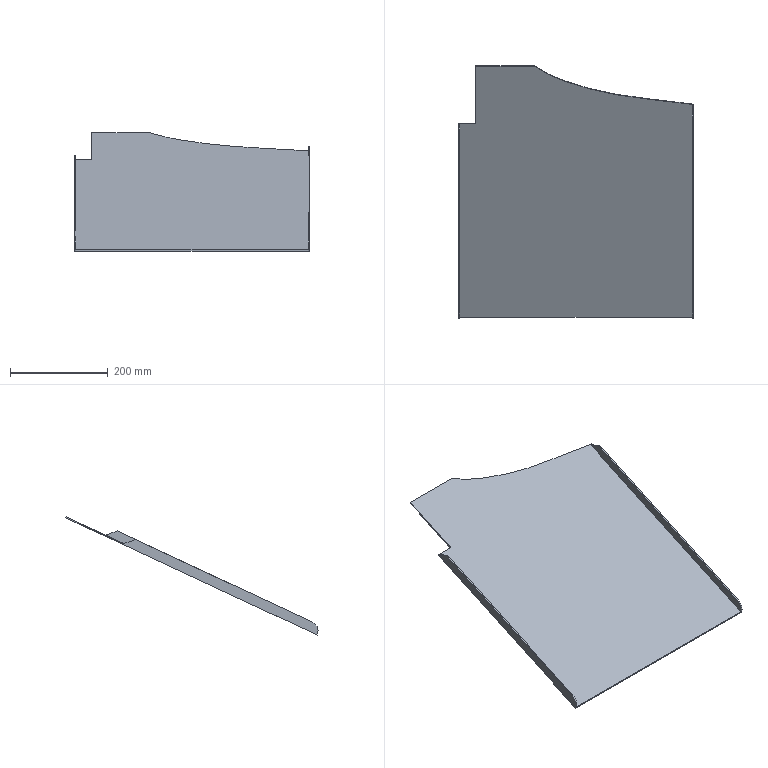Part | NX | features solid 2 | 1 solid | 17 faces | box 480 x 516.322 x 241.704 mm | volume 528303 mm3 | plane 14 | cylinder 2 | spline 1 | commonest cylinder face diameters 40 x2
STEP:
#1=CARTESIAN_POINT('',(-798.,-307.984,-104.35));
#2=VERTEX_POINT('',#1);
#3=CARTESIAN_POINT('',(-798.,-670.326,-273.313));
#4=VERTEX_POINT('',#3);
#5=CARTESIAN_POINT('',(-798.,-303.452,-102.237));
#6=DIRECTION('',(0.,-0.9063,-0.4226));
#7=VECTOR('',#6,1000.);
#8=LINE('',#5,#7);
#9=EDGE_CURVE('',#2,#4,#8,.T.);
#10=ORIENTED_EDGE('',*,*,#9,.F.);
#11=CARTESIAN_POINT('',(-800.,-307.984,-104.35));
#12=VERTEX_POINT('',#11);
#13=CARTESIAN_POINT('',(-800.,-307.984,-104.35));
#14=DIRECTION('',(1.,0.,0.));
#15=VECTOR('',#14,1000.);
#16=LINE('',#13,#15);
#17=EDGE_CURVE('',#2,#12,#16,.F.);
#18=ORIENTED_EDGE('',*,*,#17,.T.);
#19=CARTESIAN_POINT('',(-800.,-670.326,-273.313));
#20=VERTEX_POINT('',#19);
#21=CARTESIAN_POINT('',(-800.,-303.452,-102.237));
#22=DIRECTION('',(0.,-0.9063,-0.4226));
#23=VECTOR('',#22,1000.);
#24=LINE('',#21,#23);
#25=EDGE_CURVE('',#12,#20,#24,.T.);
#26=ORIENTED_EDGE('',*,*,#25,.T.);
#27=CARTESIAN_POINT('',(-800.,-670.326,-273.313));
#28=DIRECTION('',(1.,0.,0.));
#29=VECTOR('',#28,1000.);
#30=LINE('',#27,#29);
#31=EDGE_CURVE('',#20,#4,#30,.T.);
#32=ORIENTED_EDGE('',*,*,#31,.T.);
#33=EDGE_LOOP('',(#10,#18,#26,#32));
#34=FACE_BOUND('',#33,.T.);
#35=CARTESIAN_POINT('',(-800.,-303.452,-102.237));
#36=DIRECTION('',(0.,0.4226,-0.9063));
#37=DIRECTION('',(0.,-0.9063,-0.4226));
#38=AXIS2_PLACEMENT_3D('',#35,#36,#37);
#39=PLANE('',#38);
#40=ADVANCED_FACE('',(#34),#39,.F.);
#41=CARTESIAN_POINT('',(-798.,-284.063,-113.056));
#42=VERTEX_POINT('',#41);
#43=CARTESIAN_POINT('',(-798.,-680.,-297.684));
#44=VERTEX_POINT('',#43);
#45=CARTESIAN_POINT('',(-798.,-570.845,-246.785));
#46=DIRECTION('',(0.,-0.9063,-0.4226));
#47=VECTOR('',#46,1000.);
#48=LINE('',#45,#47);
#49=EDGE_CURVE('',#42,#44,#48,.T.);
#50=ORIENTED_EDGE('',*,*,#49,.F.);
#51=CARTESIAN_POINT('',(-798.,-307.984,-104.35));
#52=DIRECTION('',(0.,0.9397,-0.342));
#53=VECTOR('',#52,1000.);
#54=LINE('',#51,#53);
#55=EDGE_CURVE('',#42,#2,#54,.F.);
#56=ORIENTED_EDGE('',*,*,#55,.T.);
#57=ORIENTED_EDGE('',*,*,#9,.T.);
#58=CARTESIAN_POINT('',(-798.,-680.,-299.891));
#59=VERTEX_POINT('',#58);
#60=CARTESIAN_POINT('',(-798.,-661.874,-291.439));
#61=DIRECTION('',(-1.,0.,0.));
#62=DIRECTION('',(0.,0.,1.));
#63=AXIS2_PLACEMENT_3D('',#60,#61,#62);
#64=CIRCLE('',#63,20.);
#65=EDGE_CURVE('',#4,#59,#64,.F.);
#66=ORIENTED_EDGE('',*,*,#65,.T.);
#67=CARTESIAN_POINT('',(-798.,-680.,-430.));
#68=DIRECTION('',(0.,0.,1.));
#69=VECTOR('',#68,1000.);
#70=LINE('',#67,#69);
#71=EDGE_CURVE('',#44,#59,#70,.F.);
#72=ORIENTED_EDGE('',*,*,#71,.F.);
#73=EDGE_LOOP('',(#50,#56,#57,#66,#72));
#74=FACE_BOUND('',#73,.T.);
#75=CARTESIAN_POINT('',(-798.,-295.,-120.363));
#76=DIRECTION('',(-1.,0.,0.));
#77=DIRECTION('',(0.,0.,1.));
#78=AXIS2_PLACEMENT_3D('',#75,#76,#77);
#79=PLANE('',#78);
#80=ADVANCED_FACE('',(#74),#79,.F.);
#81=CARTESIAN_POINT('',(-765.,-166.397,-58.187));
#82=VERTEX_POINT('',#81);
#83=CARTESIAN_POINT('',(-765.,-165.552,-60.));
#84=VERTEX_POINT('',#83);
#85=CARTESIAN_POINT('',(-765.,-166.397,-58.187));
#86=DIRECTION('',(0.,0.4226,-0.9063));
#87=VECTOR('',#86,1000.);
#88=LINE('',#85,#87);
#89=EDGE_CURVE('',#82,#84,#88,.T.);
#90=ORIENTED_EDGE('',*,*,#89,.F.);
#91=CARTESIAN_POINT('',(-645.657,-166.397,-58.187));
#92=VERTEX_POINT('',#91);
#93=CARTESIAN_POINT('',(-283.631,-166.397,-58.187));
#94=DIRECTION('',(-1.,0.,0.));
#95=VECTOR('',#94,1000.);
#96=LINE('',#93,#95);
#97=EDGE_CURVE('',#92,#82,#96,.T.);
#98=ORIENTED_EDGE('',*,*,#97,.F.);
#99=CARTESIAN_POINT('',(-645.657,-165.552,-60.));
#100=VERTEX_POINT('',#99);
#101=CARTESIAN_POINT('',(-645.657,-166.397,-58.187));
#102=CARTESIAN_POINT('',(-645.657,-166.115,-58.792));
#103=CARTESIAN_POINT('',(-645.657,-165.833,-59.396));
#104=CARTESIAN_POINT('',(-645.657,-165.552,-60.));
#105=B_SPLINE_CURVE_WITH_KNOTS('',3,(#101,#102,#103,#104),.UNSPECIFIED.,.F.,.F.,(4,4),(0.,1.),.UNSPECIFIED.);
#106=EDGE_CURVE('',#92,#100,#105,.T.);
#107=ORIENTED_EDGE('',*,*,#106,.T.);
#108=CARTESIAN_POINT('',(-283.631,-165.552,-60.));
#109=DIRECTION('',(-1.,0.,0.));
#110=VECTOR('',#109,1000.);
#111=LINE('',#108,#110);
#112=EDGE_CURVE('',#100,#84,#111,.T.);
#113=ORIENTED_EDGE('',*,*,#112,.T.);
#114=EDGE_LOOP('',(#90,#98,#107,#113));
#115=FACE_BOUND('',#114,.T.);
#116=CARTESIAN_POINT('',(-283.631,-166.397,-58.187));
#117=DIRECTION('',(0.,-0.9063,-0.4226));
#118=DIRECTION('',(0.,0.4226,-0.9063));
#119=AXIS2_PLACEMENT_3D('',#116,#117,#118);
#120=PLANE('',#119);
#121=ADVANCED_FACE('',(#115),#120,.F.);
#122=CARTESIAN_POINT('',(-765.,-284.063,-113.056));
#123=VERTEX_POINT('',#122);
#124=CARTESIAN_POINT('',(-765.,-570.845,-246.785));
#125=DIRECTION('',(0.,0.9063,0.4226));
#126=VECTOR('',#125,1000.);
#127=LINE('',#124,#126);
#128=EDGE_CURVE('',#82,#123,#127,.F.);
#129=ORIENTED_EDGE('',*,*,#128,.F.);
#130=ORIENTED_EDGE('',*,*,#89,.T.);
#131=CARTESIAN_POINT('',(-765.,-283.218,-114.869));
#132=VERTEX_POINT('',#131);
#133=CARTESIAN_POINT('',(-765.,-570.,-248.597));
#134=DIRECTION('',(0.,0.9063,0.4226));
#135=VECTOR('',#134,1000.);
#136=LINE('',#133,#135);
#137=EDGE_CURVE('',#84,#132,#136,.F.);
#138=ORIENTED_EDGE('',*,*,#137,.T.);
#139=CARTESIAN_POINT('',(-765.,-284.063,-113.056));
#140=DIRECTION('',(0.,0.4226,-0.9063));
#141=VECTOR('',#140,1000.);
#142=LINE('',#139,#141);
#143=EDGE_CURVE('',#123,#132,#142,.T.);
#144=ORIENTED_EDGE('',*,*,#143,.F.);
#145=EDGE_LOOP('',(#129,#130,#138,#144));
#146=FACE_BOUND('',#145,.T.);
#147=CARTESIAN_POINT('',(-765.,-570.845,-246.785));
#148=DIRECTION('',(1.,0.,0.));
#149=DIRECTION('',(0.,0.,-1.));
#150=AXIS2_PLACEMENT_3D('',#147,#148,#149);
#151=PLANE('',#150);
#152=ADVANCED_FACE('',(#146),#151,.F.);
#153=CARTESIAN_POINT('',(-800.,-284.063,-113.056));
#154=VERTEX_POINT('',#153);
#155=CARTESIAN_POINT('',(-800.,-283.218,-114.869));
#156=VERTEX_POINT('',#155);
#157=CARTESIAN_POINT('',(-800.,-284.063,-113.056));
#158=DIRECTION('',(0.,0.4226,-0.9063));
#159=VECTOR('',#158,1000.);
#160=LINE('',#157,#159);
#161=EDGE_CURVE('',#154,#156,#160,.T.);
#162=ORIENTED_EDGE('',*,*,#161,.F.);
#163=CARTESIAN_POINT('',(-798.,-284.063,-113.056));
#164=DIRECTION('',(1.,0.,0.));
#165=VECTOR('',#164,1000.);
#166=LINE('',#163,#165);
#167=EDGE_CURVE('',#154,#42,#166,.T.);
#168=ORIENTED_EDGE('',*,*,#167,.T.);
#169=CARTESIAN_POINT('',(-800.,-284.063,-113.056));
#170=DIRECTION('',(-1.,0.,0.));
#171=VECTOR('',#170,1000.);
#172=LINE('',#169,#171);
#173=EDGE_CURVE('',#123,#42,#172,.T.);
#174=ORIENTED_EDGE('',*,*,#173,.F.);
#175=ORIENTED_EDGE('',*,*,#143,.T.);
#176=CARTESIAN_POINT('',(-800.,-283.218,-114.869));
#177=DIRECTION('',(-1.,0.,0.));
#178=VECTOR('',#177,1000.);
#179=LINE('',#176,#178);
#180=EDGE_CURVE('',#132,#156,#179,.T.);
#181=ORIENTED_EDGE('',*,*,#180,.T.);
#182=EDGE_LOOP('',(#162,#168,#174,#175,#181));
#183=FACE_BOUND('',#182,.T.);
#184=CARTESIAN_POINT('',(-800.,-284.063,-113.056));
#185=DIRECTION('',(0.,-0.9063,-0.4226));
#186=DIRECTION('',(0.,0.4226,-0.9063));
#187=AXIS2_PLACEMENT_3D('',#184,#185,#186);
#188=PLANE('',#187);
#189=ADVANCED_FACE('',(#183),#188,.F.);
#190=ORIENTED_EDGE('',*,*,#25,.F.);
#191=CARTESIAN_POINT('',(-800.,-307.984,-104.35));
#192=DIRECTION('',(0.,-0.9397,0.342));
#193=VECTOR('',#192,1000.);
#194=LINE('',#191,#193);
#195=EDGE_CURVE('',#12,#154,#194,.F.);
#196=ORIENTED_EDGE('',*,*,#195,.T.);
#197=ORIENTED_EDGE('',*,*,#161,.T.);
#198=CARTESIAN_POINT('',(-800.,-680.,-299.891));
#199=VERTEX_POINT('',#198);
#200=CARTESIAN_POINT('',(-800.,6.009,20.));
#201=DIRECTION('',(0.,-0.9063,-0.4226));
#202=VECTOR('',#201,1000.);
#203=LINE('',#200,#202);
#204=EDGE_CURVE('',#156,#199,#203,.T.);
#205=ORIENTED_EDGE('',*,*,#204,.T.);
#206=CARTESIAN_POINT('',(-800.,-661.874,-291.439));
#207=DIRECTION('',(-1.,0.,0.));
#208=DIRECTION('',(0.,0.,1.));
#209=AXIS2_PLACEMENT_3D('',#206,#207,#208);
#210=CIRCLE('',#209,20.);
#211=EDGE_CURVE('',#199,#20,#210,.T.);
#212=ORIENTED_EDGE('',*,*,#211,.T.);
#213=EDGE_LOOP('',(#190,#196,#197,#205,#212));
#214=FACE_BOUND('',#213,.T.);
#215=CARTESIAN_POINT('',(-800.,5.164,21.813));
#216=DIRECTION('',(1.,0.,0.));
#217=DIRECTION('',(0.,0.,-1.));
#218=AXIS2_PLACEMENT_3D('',#215,#216,#217);
#219=PLANE('',#218);
#220=ADVANCED_FACE('',(#214),#219,.F.);
#221=ORIENTED_EDGE('',*,*,#211,.F.);
#222=CARTESIAN_POINT('',(-800.,-680.,-299.891));
#223=DIRECTION('',(1.,0.,0.));
#224=VECTOR('',#223,1000.);
#225=LINE('',#222,#224);
#226=EDGE_CURVE('',#199,#59,#225,.T.);
#227=ORIENTED_EDGE('',*,*,#226,.T.);
#228=ORIENTED_EDGE('',*,*,#65,.F.);
#229=ORIENTED_EDGE('',*,*,#31,.F.);
#230=EDGE_LOOP('',(#221,#227,#228,#229));
#231=FACE_BOUND('',#230,.T.);
#232=CARTESIAN_POINT('',(-800.,-661.874,-291.439));
#233=DIRECTION('',(-1.,0.,0.));
#234=DIRECTION('',(0.,0.,1.));
#235=AXIS2_PLACEMENT_3D('',#232,#233,#234);
#236=CYLINDRICAL_SURFACE('',#235,20.);
#237=ADVANCED_FACE('',(#231),#236,.T.);
#238=CARTESIAN_POINT('',(-320.,-680.,-299.891));
#239=VERTEX_POINT('',#238);
#240=CARTESIAN_POINT('',(-322.,-680.,-299.891));
#241=VERTEX_POINT('',#240);
#242=CARTESIAN_POINT('',(188.564,-680.,-299.891));
#243=DIRECTION('',(1.,0.,0.));
#244=VECTOR('',#243,1000.);
#245=LINE('',#242,#244);
#246=EDGE_CURVE('',#239,#241,#245,.F.);
#247=ORIENTED_EDGE('',*,*,#246,.T.);
#248=CARTESIAN_POINT('',(188.564,-680.,-299.891));
#249=DIRECTION('',(1.,0.,0.));
#250=VECTOR('',#249,1000.);
#251=LINE('',#248,#250);
#252=EDGE_CURVE('',#241,#59,#251,.F.);
#253=ORIENTED_EDGE('',*,*,#252,.T.);
#254=ORIENTED_EDGE('',*,*,#226,.F.);
#255=ORIENTED_EDGE('',*,*,#204,.F.);
#256=ORIENTED_EDGE('',*,*,#180,.F.);
#257=ORIENTED_EDGE('',*,*,#137,.F.);
#258=ORIENTED_EDGE('',*,*,#112,.F.);
#259=CARTESIAN_POINT('',(-320.,-243.969,-96.566));
#260=VERTEX_POINT('',#259);
#261=CARTESIAN_POINT('',(-320.,-243.969,-96.566));
#262=CARTESIAN_POINT('',(-320.916,-243.837,-96.505));
#263=CARTESIAN_POINT('',(-322.075,-243.672,-96.428));
#264=CARTESIAN_POINT('',(-323.454,-243.478,-96.338));
#265=CARTESIAN_POINT('',(-324.201,-243.373,-96.289));
#266=CARTESIAN_POINT('',(-325.601,-243.178,-96.198));
#267=CARTESIAN_POINT('',(-327.59,-242.904,-96.07));
#268=CARTESIAN_POINT('',(-330.865,-242.46,-95.863));
#269=CARTESIAN_POINT('',(-335.075,-241.902,-95.603));
#270=CARTESIAN_POINT('',(-339.456,-241.337,-95.339));
#271=CARTESIAN_POINT('',(-343.061,-240.881,-95.127));
#272=CARTESIAN_POINT('',(-345.816,-240.538,-94.967));
#273=CARTESIAN_POINT('',(-348.616,-240.193,-94.806));
#274=CARTESIAN_POINT('',(-351.009,-239.902,-94.67));
#275=CARTESIAN_POINT('',(-352.672,-239.702,-94.577));
#276=CARTESIAN_POINT('',(-353.682,-239.581,-94.52));
#277=CARTESIAN_POINT('',(-354.225,-239.516,-94.49));
#278=CARTESIAN_POINT('',(-355.087,-239.413,-94.442));
#279=CARTESIAN_POINT('',(-356.418,-239.255,-94.369));
#280=CARTESIAN_POINT('',(-358.194,-239.046,-94.271));
#281=CARTESIAN_POINT('',(-362.688,-238.52,-94.026));
#282=CARTESIAN_POINT('',(-368.687,-237.828,-93.703));
#283=CARTESIAN_POINT('',(-375.598,-237.043,-93.337));
#284=CARTESIAN_POINT('',(-379.785,-236.57,-93.116));
#285=CARTESIAN_POINT('',(-382.279,-236.289,-92.985));
#286=CARTESIAN_POINT('',(-383.915,-236.105,-92.9));
#287=CARTESIAN_POINT('',(-385.188,-235.962,-92.833));
#288=CARTESIAN_POINT('',(-387.282,-235.727,-92.723));
#289=CARTESIAN_POINT('',(-391.37,-235.267,-92.509));
#290=CARTESIAN_POINT('',(-396.702,-234.665,-92.228));
#291=CARTESIAN_POINT('',(-402.356,-234.023,-91.929));
#292=CARTESIAN_POINT('',(-406.432,-233.558,-91.712));
#293=CARTESIAN_POINT('',(-409.316,-233.227,-91.558));
#294=CARTESIAN_POINT('',(-411.284,-233.,-91.452));
#295=CARTESIAN_POINT('',(-412.78,-232.826,-91.371));
#296=CARTESIAN_POINT('',(-413.651,-232.724,-91.323));
#297=CARTESIAN_POINT('',(-414.064,-232.676,-91.301));
#298=CARTESIAN_POINT('',(-414.273,-232.652,-91.289));
#299=CARTESIAN_POINT('',(-414.979,-232.569,-91.251));
#300=CARTESIAN_POINT('',(-415.686,-232.485,-91.212));
#301=CARTESIAN_POINT('',(-416.671,-232.369,-91.158));
#302=CARTESIAN_POINT('',(-418.361,-232.169,-91.064));
#303=CARTESIAN_POINT('',(-420.749,-231.884,-90.931));
#304=CARTESIAN_POINT('',(-423.553,-231.545,-90.773));
#305=CARTESIAN_POINT('',(-427.215,-231.098,-90.565));
#306=CARTESIAN_POINT('',(-431.649,-230.548,-90.308));
#307=CARTESIAN_POINT('',(-436.733,-229.901,-90.007));
#308=CARTESIAN_POINT('',(-440.383,-229.424,-89.784));
#309=CARTESIAN_POINT('',(-442.727,-229.113,-89.639));
#310=CARTESIAN_POINT('',(-443.717,-228.98,-89.577));
#311=CARTESIAN_POINT('',(-444.441,-228.883,-89.532));
#312=CARTESIAN_POINT('',(-445.383,-228.755,-89.472));
#313=CARTESIAN_POINT('',(-447.024,-228.532,-89.368));
#314=CARTESIAN_POINT('',(-449.345,-228.212,-89.219));
#315=CARTESIAN_POINT('',(-453.009,-227.698,-88.979));
#316=CARTESIAN_POINT('',(-457.497,-227.051,-88.677));
#317=CARTESIAN_POINT('',(-462.733,-226.267,-88.312));
#318=CARTESIAN_POINT('',(-466.975,-225.607,-88.004));
#319=CARTESIAN_POINT('',(-470.291,-225.077,-87.757));
#320=CARTESIAN_POINT('',(-472.749,-224.675,-87.57));
#321=CARTESIAN_POINT('',(-475.14,-224.278,-87.384));
#322=CARTESIAN_POINT('',(-478.899,-223.639,-87.087));
#323=CARTESIAN_POINT('',(-483.325,-222.86,-86.723));
#324=CARTESIAN_POINT('',(-490.377,-221.564,-86.119));
#325=CARTESIAN_POINT('',(-497.222,-220.218,-85.491));
#326=CARTESIAN_POINT('',(-503.767,-218.845,-84.851));
#327=CARTESIAN_POINT('',(-510.528,-217.362,-84.16));
#328=CARTESIAN_POINT('',(-517.355,-215.766,-83.415));
#329=CARTESIAN_POINT('',(-524.22,-214.065,-82.622));
#330=CARTESIAN_POINT('',(-528.537,-212.954,-82.104));
#331=CARTESIAN_POINT('',(-531.987,-212.043,-81.679));
#332=CARTESIAN_POINT('',(-534.621,-211.335,-81.349));
#333=CARTESIAN_POINT('',(-536.966,-210.694,-81.05));
#334=CARTESIAN_POINT('',(-540.236,-209.788,-80.628));
#335=CARTESIAN_POINT('',(-544.349,-208.623,-80.085));
#336=CARTESIAN_POINT('',(-551.093,-206.662,-79.17));
#337=CARTESIAN_POINT('',(-557.997,-204.577,-78.198));
#338=CARTESIAN_POINT('',(-565.219,-202.326,-77.148));
#339=CARTESIAN_POINT('',(-570.645,-200.582,-76.335));
#340=CARTESIAN_POINT('',(-575.821,-198.863,-75.533));
#341=CARTESIAN_POINT('',(-580.816,-197.146,-74.733));
#342=CARTESIAN_POINT('',(-584.811,-195.724,-74.069));
#343=CARTESIAN_POINT('',(-587.914,-194.588,-73.54));
#344=CARTESIAN_POINT('',(-589.805,-193.882,-73.211));
#345=CARTESIAN_POINT('',(-591.309,-193.313,-72.945));
#346=CARTESIAN_POINT('',(-592.383,-192.902,-72.754));
#347=CARTESIAN_POINT('',(-593.74,-192.378,-72.509));
#348=CARTESIAN_POINT('',(-595.434,-191.716,-72.2));
#349=CARTESIAN_POINT('',(-597.564,-190.869,-71.806));
#350=CARTESIAN_POINT('',(-602.572,-188.831,-70.855));
#351=CARTESIAN_POINT('',(-608.207,-186.401,-69.722));
#352=CARTESIAN_POINT('',(-613.586,-183.909,-68.56));
#353=CARTESIAN_POINT('',(-616.575,-182.475,-67.891));
#354=CARTESIAN_POINT('',(-618.439,-181.557,-67.463));
#355=CARTESIAN_POINT('',(-619.85,-180.851,-67.134));
#356=CARTESIAN_POINT('',(-621.541,-179.992,-66.734));
#357=CARTESIAN_POINT('',(-624.33,-178.545,-66.059));
#358=CARTESIAN_POINT('',(-629.873,-175.548,-64.662));
#359=CARTESIAN_POINT('',(-637.361,-171.14,-62.606));
#360=CARTESIAN_POINT('',(-642.96,-167.441,-60.881));
#361=CARTESIAN_POINT('',(-645.657,-165.552,-60.));
#362=B_SPLINE_CURVE_WITH_KNOTS('',3,(#261,#262,#263,#264,#265,#266,#267,#268,#269,#270,#271,#272,#273,#274,#275,#276,#277,#278,#279,#280,#281,#282,#283,#284,#285,#286,#287,#288,#289,#290,#291,#292,#293,#294,#295,#296,#297,#298,#299,#300,#301,#302,#303,#304,#305,#306,#307,#308,#309,#310,#311,#312,#313,#314,#315,#316,#317,#318,#319,#320,#321,#322,#323,#324,#325,#326,#327,#328,#329,#330,#331,#332,#333,#334,#335,#336,#337,#338,#339,#340,#341,#342,#343,#344,#345,#346,#347,#348,#349,#350,#351,#352,#353,#354,#355,#356,#357,#358,#359,#360,#361),.UNSPECIFIED.,.F.,.F.,(4,1,1,1,1,1,1,1,1,1,1,1,1,1,1,1,1,1,1,1,1,1,1,1,1,1,1,1,1,1,1,1,1,1,1,1,1,1,1,1,1,1,1,1,1,1,1,1,1,1,1,1,1,1,1,1,1,1,1,1,1,1,1,1,1,1,1,1,1,1,1,1,1,1,1,1,1,1,1,1,1,1,1,1,1,1,1,1,1,1,1,1,1,1,1,1,1,1,4),(0.653,0.6557,0.6564,0.6571,0.6584,0.6612,0.6639,0.6693,0.6747,0.6774,0.6801,0.6828,0.6856,0.6869,0.6876,0.6883,0.6896,0.691,0.6937,0.6964,0.7072,0.7127,0.7154,0.7181,0.7188,0.7194,0.7208,0.7235,0.7289,0.7343,0.7398,0.7425,0.7452,0.7479,0.7493,0.7496,0.7499,0.7506,0.7513,0.752,0.7533,0.756,0.7587,0.7615,0.7669,0.7723,0.7777,0.7791,0.7804,0.7811,0.7818,0.7831,0.7859,0.7886,0.794,0.7994,0.8048,0.8075,0.8102,0.813,0.8157,0.8211,0.8265,0.8374,0.8428,0.8482,0.859,0.8645,0.8699,0.8726,0.8753,0.878,0.8807,0.8861,0.8916,0.9024,0.9078,0.9133,0.9187,0.9241,0.9295,0.9322,0.9349,0.9363,0.9377,0.939,0.9404,0.9431,0.9458,0.9566,0.962,0.9648,0.9675,0.9688,0.9702,0.9729,0.9783,0.9892,1.),.UNSPECIFIED.);
#363=EDGE_CURVE('',#260,#100,#362,.T.);
#364=ORIENTED_EDGE('',*,*,#363,.F.);
#365=CARTESIAN_POINT('',(-320.,-570.,-248.597));
#366=DIRECTION('',(0.,-0.9063,-0.4226));
#367=VECTOR('',#366,1000.);
#368=LINE('',#365,#367);
#369=EDGE_CURVE('',#260,#239,#368,.T.);
#370=ORIENTED_EDGE('',*,*,#369,.T.);
#371=EDGE_LOOP('',(#247,#253,#254,#255,#256,#257,#258,#364,#370));
#372=FACE_BOUND('',#371,.T.);
#373=CARTESIAN_POINT('',(-800.,-570.,-248.597));
#374=DIRECTION('',(0.,-0.4226,0.9063));
#375=DIRECTION('',(0.,-0.9063,-0.4226));
#376=AXIS2_PLACEMENT_3D('',#373,#374,#375);
#377=PLANE('',#376);
#378=ADVANCED_FACE('',(#372),#377,.F.);
#379=CARTESIAN_POINT('',(-320.,-244.814,-94.754));
#380=VERTEX_POINT('',#379);
#381=CARTESIAN_POINT('',(-320.,-244.814,-94.754));
#382=CARTESIAN_POINT('',(-320.916,-244.682,-94.692));
#383=CARTESIAN_POINT('',(-322.075,-244.517,-94.615));
#384=CARTESIAN_POINT('',(-323.454,-244.323,-94.525));
#385=CARTESIAN_POINT('',(-324.201,-244.219,-94.476));
#386=CARTESIAN_POINT('',(-325.601,-244.023,-94.385));
#387=CARTESIAN_POINT('',(-327.59,-243.749,-94.257));
#388=CARTESIAN_POINT('',(-330.865,-243.305,-94.05));
#389=CARTESIAN_POINT('',(-335.075,-242.747,-93.79));
#390=CARTESIAN_POINT('',(-339.456,-242.182,-93.527));
#391=CARTESIAN_POINT('',(-343.061,-241.727,-93.314));
#392=CARTESIAN_POINT('',(-345.816,-241.383,-93.154));
#393=CARTESIAN_POINT('',(-348.616,-241.038,-92.993));
#394=CARTESIAN_POINT('',(-351.009,-240.748,-92.858));
#395=CARTESIAN_POINT('',(-352.672,-240.547,-92.764));
#396=CARTESIAN_POINT('',(-353.682,-240.426,-92.708));
#397=CARTESIAN_POINT('',(-354.225,-240.361,-92.678));
#398=CARTESIAN_POINT('',(-355.087,-240.258,-92.63));
#399=CARTESIAN_POINT('',(-356.418,-240.101,-92.556));
#400=CARTESIAN_POINT('',(-358.194,-239.891,-92.458));
#401=CARTESIAN_POINT('',(-362.688,-239.365,-92.213));
#402=CARTESIAN_POINT('',(-368.687,-238.673,-91.89));
#403=CARTESIAN_POINT('',(-375.598,-237.888,-91.524));
#404=CARTESIAN_POINT('',(-379.785,-237.415,-91.304));
#405=CARTESIAN_POINT('',(-382.279,-237.134,-91.173));
#406=CARTESIAN_POINT('',(-383.915,-236.95,-91.087));
#407=CARTESIAN_POINT('',(-385.188,-236.807,-91.02));
#408=CARTESIAN_POINT('',(-387.282,-236.572,-90.911));
#409=CARTESIAN_POINT('',(-391.37,-236.112,-90.696));
#410=CARTESIAN_POINT('',(-396.702,-235.51,-90.415));
#411=CARTESIAN_POINT('',(-402.356,-234.869,-90.116));
#412=CARTESIAN_POINT('',(-406.432,-234.403,-89.899));
#413=CARTESIAN_POINT('',(-409.316,-234.072,-89.745));
#414=CARTESIAN_POINT('',(-411.284,-233.845,-89.639));
#415=CARTESIAN_POINT('',(-412.78,-233.671,-89.558));
#416=CARTESIAN_POINT('',(-413.651,-233.57,-89.511));
#417=CARTESIAN_POINT('',(-414.064,-233.521,-89.488));
#418=CARTESIAN_POINT('',(-414.273,-233.497,-89.477));
#419=CARTESIAN_POINT('',(-414.979,-233.414,-89.438));
#420=CARTESIAN_POINT('',(-415.686,-233.331,-89.399));
#421=CARTESIAN_POINT('',(-416.671,-233.214,-89.345));
#422=CARTESIAN_POINT('',(-418.361,-233.014,-89.252));
#423=CARTESIAN_POINT('',(-420.749,-232.729,-89.119));
#424=CARTESIAN_POINT('',(-423.553,-232.391,-88.961));
#425=CARTESIAN_POINT('',(-427.215,-231.944,-88.752));
#426=CARTESIAN_POINT('',(-431.649,-231.393,-88.496));
#427=CARTESIAN_POINT('',(-436.733,-230.746,-88.194));
#428=CARTESIAN_POINT('',(-440.383,-230.269,-87.972));
#429=CARTESIAN_POINT('',(-442.727,-229.958,-87.826));
#430=CARTESIAN_POINT('',(-443.717,-229.825,-87.765));
#431=CARTESIAN_POINT('',(-444.441,-229.728,-87.719));
#432=CARTESIAN_POINT('',(-445.383,-229.601,-87.66));
#433=CARTESIAN_POINT('',(-447.024,-229.377,-87.556));
#434=CARTESIAN_POINT('',(-449.345,-229.058,-87.407));
#435=CARTESIAN_POINT('',(-453.009,-228.543,-87.167));
#436=CARTESIAN_POINT('',(-457.497,-227.896,-86.865));
#437=CARTESIAN_POINT('',(-462.733,-227.112,-86.499));
#438=CARTESIAN_POINT('',(-466.975,-226.453,-86.192));
#439=CARTESIAN_POINT('',(-470.291,-225.922,-85.944));
#440=CARTESIAN_POINT('',(-472.749,-225.521,-85.757));
#441=CARTESIAN_POINT('',(-475.14,-225.123,-85.572));
#442=CARTESIAN_POINT('',(-478.899,-224.484,-85.274));
#443=CARTESIAN_POINT('',(-483.325,-223.705,-84.911));
#444=CARTESIAN_POINT('',(-490.377,-222.409,-84.306));
#445=CARTESIAN_POINT('',(-497.222,-221.063,-83.679));
#446=CARTESIAN_POINT('',(-503.767,-219.69,-83.038));
#447=CARTESIAN_POINT('',(-510.528,-218.207,-82.347));
#448=CARTESIAN_POINT('',(-517.355,-216.611,-81.603));
#449=CARTESIAN_POINT('',(-524.22,-214.91,-80.809));
#450=CARTESIAN_POINT('',(-528.537,-213.799,-80.292));
#451=CARTESIAN_POINT('',(-531.987,-212.888,-79.867));
#452=CARTESIAN_POINT('',(-534.621,-212.18,-79.536));
#453=CARTESIAN_POINT('',(-536.966,-211.539,-79.238));
#454=CARTESIAN_POINT('',(-540.236,-210.633,-78.815));
#455=CARTESIAN_POINT('',(-544.349,-209.469,-78.272));
#456=CARTESIAN_POINT('',(-551.093,-207.507,-77.357));
#457=CARTESIAN_POINT('',(-557.997,-205.422,-76.385));
#458=CARTESIAN_POINT('',(-565.219,-203.171,-75.335));
#459=CARTESIAN_POINT('',(-570.645,-201.427,-74.522));
#460=CARTESIAN_POINT('',(-575.821,-199.708,-73.721));
#461=CARTESIAN_POINT('',(-580.816,-197.992,-72.92));
#462=CARTESIAN_POINT('',(-584.811,-196.569,-72.257));
#463=CARTESIAN_POINT('',(-587.914,-195.433,-71.727));
#464=CARTESIAN_POINT('',(-589.805,-194.727,-71.398));
#465=CARTESIAN_POINT('',(-591.309,-194.158,-71.133));
#466=CARTESIAN_POINT('',(-592.383,-193.748,-70.941));
#467=CARTESIAN_POINT('',(-593.74,-193.224,-70.697));
#468=CARTESIAN_POINT('',(-595.434,-192.561,-70.388));
#469=CARTESIAN_POINT('',(-597.564,-191.714,-69.993));
#470=CARTESIAN_POINT('',(-602.572,-189.676,-69.043));
#471=CARTESIAN_POINT('',(-608.207,-187.246,-67.91));
#472=CARTESIAN_POINT('',(-613.586,-184.755,-66.748));
#473=CARTESIAN_POINT('',(-616.575,-183.32,-66.079));
#474=CARTESIAN_POINT('',(-618.439,-182.402,-65.651));
#475=CARTESIAN_POINT('',(-619.85,-181.696,-65.321));
#476=CARTESIAN_POINT('',(-621.541,-180.838,-64.921));
#477=CARTESIAN_POINT('',(-624.33,-179.39,-64.246));
#478=CARTESIAN_POINT('',(-629.873,-176.394,-62.849));
#479=CARTESIAN_POINT('',(-637.361,-171.985,-60.793));
#480=CARTESIAN_POINT('',(-642.96,-168.286,-59.068));
#481=CARTESIAN_POINT('',(-645.657,-166.397,-58.187));
#482=B_SPLINE_CURVE_WITH_KNOTS('',3,(#381,#382,#383,#384,#385,#386,#387,#388,#389,#390,#391,#392,#393,#394,#395,#396,#397,#398,#399,#400,#401,#402,#403,#404,#405,#406,#407,#408,#409,#410,#411,#412,#413,#414,#415,#416,#417,#418,#419,#420,#421,#422,#423,#424,#425,#426,#427,#428,#429,#430,#431,#432,#433,#434,#435,#436,#437,#438,#439,#440,#441,#442,#443,#444,#445,#446,#447,#448,#449,#450,#451,#452,#453,#454,#455,#456,#457,#458,#459,#460,#461,#462,#463,#464,#465,#466,#467,#468,#469,#470,#471,#472,#473,#474,#475,#476,#477,#478,#479,#480,#481),.UNSPECIFIED.,.F.,.F.,(4,1,1,1,1,1,1,1,1,1,1,1,1,1,1,1,1,1,1,1,1,1,1,1,1,1,1,1,1,1,1,1,1,1,1,1,1,1,1,1,1,1,1,1,1,1,1,1,1,1,1,1,1,1,1,1,1,1,1,1,1,1,1,1,1,1,1,1,1,1,1,1,1,1,1,1,1,1,1,1,1,1,1,1,1,1,1,1,1,1,1,1,1,1,1,1,1,1,4),(0.653,0.6557,0.6564,0.6571,0.6584,0.6612,0.6639,0.6693,0.6747,0.6774,0.6801,0.6828,0.6856,0.6869,0.6876,0.6883,0.6896,0.691,0.6937,0.6964,0.7072,0.7127,0.7154,0.7181,0.7188,0.7194,0.7208,0.7235,0.7289,0.7343,0.7398,0.7425,0.7452,0.7479,0.7493,0.7496,0.7499,0.7506,0.7513,0.752,0.7533,0.756,0.7587,0.7615,0.7669,0.7723,0.7777,0.7791,0.7804,0.7811,0.7818,0.7831,0.7859,0.7886,0.794,0.7994,0.8048,0.8075,0.8102,0.813,0.8157,0.8211,0.8265,0.8374,0.8428,0.8482,0.859,0.8645,0.8699,0.8726,0.8753,0.878,0.8807,0.8861,0.8916,0.9024,0.9078,0.9133,0.9187,0.9241,0.9295,0.9322,0.9349,0.9363,0.9377,0.939,0.9404,0.9431,0.9458,0.9566,0.962,0.9648,0.9675,0.9688,0.9702,0.9729,0.9783,0.9892,1.),.UNSPECIFIED.);
#483=EDGE_CURVE('',#380,#92,#482,.T.);
#484=ORIENTED_EDGE('',*,*,#483,.F.);
#485=CARTESIAN_POINT('',(-320.,-244.814,-94.754));
#486=DIRECTION('',(0.,0.4226,-0.9063));
#487=VECTOR('',#486,1000.);
#488=LINE('',#485,#487);
#489=EDGE_CURVE('',#380,#260,#488,.T.);
#490=ORIENTED_EDGE('',*,*,#489,.T.);
#491=ORIENTED_EDGE('',*,*,#363,.T.);
#492=ORIENTED_EDGE('',*,*,#106,.F.);
#493=EDGE_LOOP('',(#484,#490,#491,#492));
#494=FACE_BOUND('',#493,.T.);
#495=CARTESIAN_POINT('',(-320.,-244.814,-94.754));
#496=CARTESIAN_POINT('',(-320.,-243.969,-96.566));
#497=CARTESIAN_POINT('',(-320.916,-244.682,-94.692));
#498=CARTESIAN_POINT('',(-320.916,-243.837,-96.505));
#499=CARTESIAN_POINT('',(-322.075,-244.517,-94.615));
#500=CARTESIAN_POINT('',(-322.075,-243.672,-96.428));
#501=CARTESIAN_POINT('',(-323.454,-244.323,-94.525));
#502=CARTESIAN_POINT('',(-323.454,-243.478,-96.338));
#503=CARTESIAN_POINT('',(-324.201,-244.219,-94.476));
#504=CARTESIAN_POINT('',(-324.201,-243.373,-96.289));
#505=CARTESIAN_POINT('',(-325.601,-244.023,-94.385));
#506=CARTESIAN_POINT('',(-325.601,-243.178,-96.198));
#507=CARTESIAN_POINT('',(-327.59,-243.749,-94.257));
#508=CARTESIAN_POINT('',(-327.59,-242.904,-96.07));
#509=CARTESIAN_POINT('',(-330.865,-243.305,-94.05));
#510=CARTESIAN_POINT('',(-330.865,-242.46,-95.863));
#511=CARTESIAN_POINT('',(-335.075,-242.747,-93.79));
#512=CARTESIAN_POINT('',(-335.075,-241.902,-95.603));
#513=CARTESIAN_POINT('',(-339.456,-242.182,-93.527));
#514=CARTESIAN_POINT('',(-339.456,-241.337,-95.339));
#515=CARTESIAN_POINT('',(-343.061,-241.727,-93.314));
#516=CARTESIAN_POINT('',(-343.061,-240.881,-95.127));
#517=CARTESIAN_POINT('',(-345.816,-241.383,-93.154));
#518=CARTESIAN_POINT('',(-345.816,-240.538,-94.967));
#519=CARTESIAN_POINT('',(-348.616,-241.038,-92.993));
#520=CARTESIAN_POINT('',(-348.616,-240.193,-94.806));
#521=CARTESIAN_POINT('',(-351.009,-240.748,-92.858));
#522=CARTESIAN_POINT('',(-351.009,-239.902,-94.67));
#523=CARTESIAN_POINT('',(-352.672,-240.547,-92.764));
#524=CARTESIAN_POINT('',(-352.672,-239.702,-94.577));
#525=CARTESIAN_POINT('',(-353.682,-240.426,-92.708));
#526=CARTESIAN_POINT('',(-353.682,-239.581,-94.52));
#527=CARTESIAN_POINT('',(-354.225,-240.361,-92.678));
#528=CARTESIAN_POINT('',(-354.225,-239.516,-94.49));
#529=CARTESIAN_POINT('',(-355.087,-240.258,-92.63));
#530=CARTESIAN_POINT('',(-355.087,-239.413,-94.442));
#531=CARTESIAN_POINT('',(-356.418,-240.101,-92.556));
#532=CARTESIAN_POINT('',(-356.418,-239.255,-94.369));
#533=CARTESIAN_POINT('',(-358.194,-239.891,-92.458));
#534=CARTESIAN_POINT('',(-358.194,-239.046,-94.271));
#535=CARTESIAN_POINT('',(-362.688,-239.365,-92.213));
#536=CARTESIAN_POINT('',(-362.688,-238.52,-94.026));
#537=CARTESIAN_POINT('',(-368.687,-238.673,-91.89));
#538=CARTESIAN_POINT('',(-368.687,-237.828,-93.703));
#539=CARTESIAN_POINT('',(-375.598,-237.888,-91.524));
#540=CARTESIAN_POINT('',(-375.598,-237.043,-93.337));
#541=CARTESIAN_POINT('',(-379.785,-237.415,-91.304));
#542=CARTESIAN_POINT('',(-379.785,-236.57,-93.116));
#543=CARTESIAN_POINT('',(-382.279,-237.134,-91.173));
#544=CARTESIAN_POINT('',(-382.279,-236.289,-92.985));
#545=CARTESIAN_POINT('',(-383.915,-236.95,-91.087));
#546=CARTESIAN_POINT('',(-383.915,-236.105,-92.9));
#547=CARTESIAN_POINT('',(-385.188,-236.807,-91.02));
#548=CARTESIAN_POINT('',(-385.188,-235.962,-92.833));
#549=CARTESIAN_POINT('',(-387.282,-236.572,-90.911));
#550=CARTESIAN_POINT('',(-387.282,-235.727,-92.723));
#551=CARTESIAN_POINT('',(-391.37,-236.112,-90.696));
#552=CARTESIAN_POINT('',(-391.37,-235.267,-92.509));
#553=CARTESIAN_POINT('',(-396.702,-235.51,-90.415));
#554=CARTESIAN_POINT('',(-396.702,-234.665,-92.228));
#555=CARTESIAN_POINT('',(-402.356,-234.869,-90.116));
#556=CARTESIAN_POINT('',(-402.356,-234.023,-91.929));
#557=CARTESIAN_POINT('',(-406.432,-234.403,-89.899));
#558=CARTESIAN_POINT('',(-406.432,-233.558,-91.712));
#559=CARTESIAN_POINT('',(-409.316,-234.072,-89.745));
#560=CARTESIAN_POINT('',(-409.316,-233.227,-91.558));
#561=CARTESIAN_POINT('',(-411.284,-233.845,-89.639));
#562=CARTESIAN_POINT('',(-411.284,-233.,-91.452));
#563=CARTESIAN_POINT('',(-412.78,-233.671,-89.558));
#564=CARTESIAN_POINT('',(-412.78,-232.826,-91.371));
#565=CARTESIAN_POINT('',(-413.651,-233.57,-89.511));
#566=CARTESIAN_POINT('',(-413.651,-232.724,-91.323));
#567=CARTESIAN_POINT('',(-414.064,-233.521,-89.488));
#568=CARTESIAN_POINT('',(-414.064,-232.676,-91.301));
#569=CARTESIAN_POINT('',(-414.273,-233.497,-89.477));
#570=CARTESIAN_POINT('',(-414.273,-232.652,-91.289));
#571=CARTESIAN_POINT('',(-414.979,-233.414,-89.438));
#572=CARTESIAN_POINT('',(-414.979,-232.569,-91.251));
#573=CARTESIAN_POINT('',(-415.686,-233.331,-89.399));
#574=CARTESIAN_POINT('',(-415.686,-232.485,-91.212));
#575=CARTESIAN_POINT('',(-416.671,-233.214,-89.345));
#576=CARTESIAN_POINT('',(-416.671,-232.369,-91.158));
#577=CARTESIAN_POINT('',(-418.361,-233.014,-89.252));
#578=CARTESIAN_POINT('',(-418.361,-232.169,-91.064));
#579=CARTESIAN_POINT('',(-420.749,-232.729,-89.119));
#580=CARTESIAN_POINT('',(-420.749,-231.884,-90.931));
#581=CARTESIAN_POINT('',(-423.553,-232.391,-88.961));
#582=CARTESIAN_POINT('',(-423.553,-231.545,-90.773));
#583=CARTESIAN_POINT('',(-427.215,-231.944,-88.752));
#584=CARTESIAN_POINT('',(-427.215,-231.098,-90.565));
#585=CARTESIAN_POINT('',(-431.649,-231.393,-88.496));
#586=CARTESIAN_POINT('',(-431.649,-230.548,-90.308));
#587=CARTESIAN_POINT('',(-436.733,-230.746,-88.194));
#588=CARTESIAN_POINT('',(-436.733,-229.901,-90.007));
#589=CARTESIAN_POINT('',(-440.383,-230.269,-87.972));
#590=CARTESIAN_POINT('',(-440.383,-229.424,-89.784));
#591=CARTESIAN_POINT('',(-442.727,-229.958,-87.826));
#592=CARTESIAN_POINT('',(-442.727,-229.113,-89.639));
#593=CARTESIAN_POINT('',(-443.717,-229.825,-87.765));
#594=CARTESIAN_POINT('',(-443.717,-228.98,-89.577));
#595=CARTESIAN_POINT('',(-444.441,-229.728,-87.719));
#596=CARTESIAN_POINT('',(-444.441,-228.883,-89.532));
#597=CARTESIAN_POINT('',(-445.383,-229.601,-87.66));
#598=CARTESIAN_POINT('',(-445.383,-228.755,-89.472));
#599=CARTESIAN_POINT('',(-447.024,-229.377,-87.556));
#600=CARTESIAN_POINT('',(-447.024,-228.532,-89.368));
#601=CARTESIAN_POINT('',(-449.345,-229.058,-87.407));
#602=CARTESIAN_POINT('',(-449.345,-228.212,-89.219));
#603=CARTESIAN_POINT('',(-453.009,-228.543,-87.167));
#604=CARTESIAN_POINT('',(-453.009,-227.698,-88.979));
#605=CARTESIAN_POINT('',(-457.497,-227.896,-86.865));
#606=CARTESIAN_POINT('',(-457.497,-227.051,-88.677));
#607=CARTESIAN_POINT('',(-462.733,-227.112,-86.499));
#608=CARTESIAN_POINT('',(-462.733,-226.267,-88.312));
#609=CARTESIAN_POINT('',(-466.975,-226.453,-86.192));
#610=CARTESIAN_POINT('',(-466.975,-225.607,-88.004));
#611=CARTESIAN_POINT('',(-470.291,-225.922,-85.944));
#612=CARTESIAN_POINT('',(-470.291,-225.077,-87.757));
#613=CARTESIAN_POINT('',(-472.749,-225.521,-85.757));
#614=CARTESIAN_POINT('',(-472.749,-224.675,-87.57));
#615=CARTESIAN_POINT('',(-475.14,-225.123,-85.572));
#616=CARTESIAN_POINT('',(-475.14,-224.278,-87.384));
#617=CARTESIAN_POINT('',(-478.899,-224.484,-85.274));
#618=CARTESIAN_POINT('',(-478.899,-223.639,-87.087));
#619=CARTESIAN_POINT('',(-483.325,-223.705,-84.911));
#620=CARTESIAN_POINT('',(-483.325,-222.86,-86.723));
#621=CARTESIAN_POINT('',(-490.377,-222.409,-84.306));
#622=CARTESIAN_POINT('',(-490.377,-221.564,-86.119));
#623=CARTESIAN_POINT('',(-497.222,-221.063,-83.679));
#624=CARTESIAN_POINT('',(-497.222,-220.218,-85.491));
#625=CARTESIAN_POINT('',(-503.767,-219.69,-83.038));
#626=CARTESIAN_POINT('',(-503.767,-218.845,-84.851));
#627=CARTESIAN_POINT('',(-510.528,-218.207,-82.347));
#628=CARTESIAN_POINT('',(-510.528,-217.362,-84.16));
#629=CARTESIAN_POINT('',(-517.355,-216.611,-81.603));
#630=CARTESIAN_POINT('',(-517.355,-215.766,-83.415));
#631=CARTESIAN_POINT('',(-524.22,-214.91,-80.809));
#632=CARTESIAN_POINT('',(-524.22,-214.065,-82.622));
#633=CARTESIAN_POINT('',(-528.537,-213.799,-80.292));
#634=CARTESIAN_POINT('',(-528.537,-212.954,-82.104));
#635=CARTESIAN_POINT('',(-531.987,-212.888,-79.867));
#636=CARTESIAN_POINT('',(-531.987,-212.043,-81.679));
#637=CARTESIAN_POINT('',(-534.621,-212.18,-79.536));
#638=CARTESIAN_POINT('',(-534.621,-211.335,-81.349));
#639=CARTESIAN_POINT('',(-536.966,-211.539,-79.238));
#640=CARTESIAN_POINT('',(-536.966,-210.694,-81.05));
#641=CARTESIAN_POINT('',(-540.236,-210.633,-78.815));
#642=CARTESIAN_POINT('',(-540.236,-209.788,-80.628));
#643=CARTESIAN_POINT('',(-544.349,-209.469,-78.272));
#644=CARTESIAN_POINT('',(-544.349,-208.623,-80.085));
#645=CARTESIAN_POINT('',(-551.093,-207.507,-77.357));
#646=CARTESIAN_POINT('',(-551.093,-206.662,-79.17));
#647=CARTESIAN_POINT('',(-557.997,-205.422,-76.385));
#648=CARTESIAN_POINT('',(-557.997,-204.577,-78.198));
#649=CARTESIAN_POINT('',(-565.219,-203.171,-75.335));
#650=CARTESIAN_POINT('',(-565.219,-202.326,-77.148));
#651=CARTESIAN_POINT('',(-570.645,-201.427,-74.522));
#652=CARTESIAN_POINT('',(-570.645,-200.582,-76.335));
#653=CARTESIAN_POINT('',(-575.821,-199.708,-73.721));
#654=CARTESIAN_POINT('',(-575.821,-198.863,-75.533));
#655=CARTESIAN_POINT('',(-580.816,-197.992,-72.92));
#656=CARTESIAN_POINT('',(-580.816,-197.146,-74.733));
#657=CARTESIAN_POINT('',(-584.811,-196.569,-72.257));
#658=CARTESIAN_POINT('',(-584.811,-195.724,-74.069));
#659=CARTESIAN_POINT('',(-587.914,-195.433,-71.727));
#660=CARTESIAN_POINT('',(-587.914,-194.588,-73.54));
#661=CARTESIAN_POINT('',(-589.805,-194.727,-71.398));
#662=CARTESIAN_POINT('',(-589.805,-193.882,-73.211));
#663=CARTESIAN_POINT('',(-591.309,-194.158,-71.133));
#664=CARTESIAN_POINT('',(-591.309,-193.313,-72.945));
#665=CARTESIAN_POINT('',(-592.383,-193.748,-70.941));
#666=CARTESIAN_POINT('',(-592.383,-192.902,-72.754));
#667=CARTESIAN_POINT('',(-593.74,-193.224,-70.697));
#668=CARTESIAN_POINT('',(-593.74,-192.378,-72.509));
#669=CARTESIAN_POINT('',(-595.434,-192.561,-70.388));
#670=CARTESIAN_POINT('',(-595.434,-191.716,-72.2));
#671=CARTESIAN_POINT('',(-597.564,-191.714,-69.993));
#672=CARTESIAN_POINT('',(-597.564,-190.869,-71.806));
#673=CARTESIAN_POINT('',(-602.572,-189.676,-69.043));
#674=CARTESIAN_POINT('',(-602.572,-188.831,-70.855));
#675=CARTESIAN_POINT('',(-608.207,-187.246,-67.91));
#676=CARTESIAN_POINT('',(-608.207,-186.401,-69.722));
#677=CARTESIAN_POINT('',(-613.586,-184.755,-66.748));
#678=CARTESIAN_POINT('',(-613.586,-183.909,-68.56));
#679=CARTESIAN_POINT('',(-616.575,-183.32,-66.079));
#680=CARTESIAN_POINT('',(-616.575,-182.475,-67.891));
#681=CARTESIAN_POINT('',(-618.439,-182.402,-65.651));
#682=CARTESIAN_POINT('',(-618.439,-181.557,-67.463));
#683=CARTESIAN_POINT('',(-619.85,-181.696,-65.321));
#684=CARTESIAN_POINT('',(-619.85,-180.851,-67.134));
#685=CARTESIAN_POINT('',(-621.541,-180.838,-64.921));
#686=CARTESIAN_POINT('',(-621.541,-179.992,-66.734));
#687=CARTESIAN_POINT('',(-624.33,-179.39,-64.246));
#688=CARTESIAN_POINT('',(-624.33,-178.545,-66.059));
#689=CARTESIAN_POINT('',(-629.873,-176.394,-62.849));
#690=CARTESIAN_POINT('',(-629.873,-175.548,-64.662));
#691=CARTESIAN_POINT('',(-637.361,-171.985,-60.793));
#692=CARTESIAN_POINT('',(-637.361,-171.14,-62.606));
#693=CARTESIAN_POINT('',(-642.96,-168.286,-59.068));
#694=CARTESIAN_POINT('',(-642.96,-167.441,-60.881));
#695=CARTESIAN_POINT('',(-645.657,-166.397,-58.187));
#696=CARTESIAN_POINT('',(-645.657,-165.552,-60.));
#697=B_SPLINE_SURFACE_WITH_KNOTS('',3,1,((#495,#496),(#497,#498),(#499,#500),(#501,#502),(#503,#504),(#505,#506),(#507,#508),(#509,#510),(#511,#512),(#513,#514),(#515,#516),(#517,#518),(#519,#520),(#521,#522),(#523,#524),(#525,#526),(#527,#528),(#529,#530),(#531,#532),(#533,#534),(#535,#536),(#537,#538),(#539,#540),(#541,#542),(#543,#544),(#545,#546),(#547,#548),(#549,#550),(#551,#552),(#553,#554),(#555,#556),(#557,#558),(#559,#560),(#561,#562),(#563,#564),(#565,#566),(#567,#568),(#569,#570),(#571,#572),(#573,#574),(#575,#576),(#577,#578),(#579,#580),(#581,#582),(#583,#584),(#585,#586),(#587,#588),(#589,#590),(#591,#592),(#593,#594),(#595,#596),(#597,#598),(#599,#600),(#601,#602),(#603,#604),(#605,#606),(#607,#608),(#609,#610),(#611,#612),(#613,#614),(#615,#616),(#617,#618),(#619,#620),(#621,#622),(#623,#624),(#625,#626),(#627,#628),(#629,#630),(#631,#632),(#633,#634),(#635,#636),(#637,#638),(#639,#640),(#641,#642),(#643,#644),(#645,#646),(#647,#648),(#649,#650),(#651,#652),(#653,#654),(#655,#656),(#657,#658),(#659,#660),(#661,#662),(#663,#664),(#665,#666),(#667,#668),(#669,#670),(#671,#672),(#673,#674),(#675,#676),(#677,#678),(#679,#680),(#681,#682),(#683,#684),(#685,#686),(#687,#688),(#689,#690),(#691,#692),(#693,#694),(#695,#696)),.SURF_OF_LINEAR_EXTRUSION.,.F.,.F.,.F.,(4,1,1,1,1,1,1,1,1,1,1,1,1,1,1,1,1,1,1,1,1,1,1,1,1,1,1,1,1,1,1,1,1,1,1,1,1,1,1,1,1,1,1,1,1,1,1,1,1,1,1,1,1,1,1,1,1,1,1,1,1,1,1,1,1,1,1,1,1,1,1,1,1,1,1,1,1,1,1,1,1,1,1,1,1,1,1,1,1,1,1,1,1,1,1,1,1,1,4),(2,2),(0.653,0.6557,0.6564,0.6571,0.6584,0.6612,0.6639,0.6693,0.6747,0.6774,0.6801,0.6828,0.6856,0.6869,0.6876,0.6883,0.6896,0.691,0.6937,0.6964,0.7072,0.7127,0.7154,0.7181,0.7188,0.7194,0.7208,0.7235,0.7289,0.7343,0.7398,0.7425,0.7452,0.7479,0.7493,0.7496,0.7499,0.7506,0.7513,0.752,0.7533,0.756,0.7587,0.7615,0.7669,0.7723,0.7777,0.7791,0.7804,0.7811,0.7818,0.7831,0.7859,0.7886,0.794,0.7994,0.8048,0.8075,0.8102,0.813,0.8157,0.8211,0.8265,0.8374,0.8428,0.8482,0.859,0.8645,0.8699,0.8726,0.8753,0.878,0.8807,0.8861,0.8916,0.9024,0.9078,0.9133,0.9187,0.9241,0.9295,0.9322,0.9349,0.9363,0.9377,0.939,0.9404,0.9431,0.9458,0.9566,0.962,0.9648,0.9675,0.9688,0.9702,0.9729,0.9783,0.9892,1.),(0.,1.),.UNSPECIFIED.);
#698=ADVANCED_FACE('',(#494),#697,.F.);
#699=CARTESIAN_POINT('',(-322.,-246.626,-95.599));
#700=VERTEX_POINT('',#699);
#701=CARTESIAN_POINT('',(-322.,-680.,-297.684));
#702=VERTEX_POINT('',#701);
#703=CARTESIAN_POINT('',(-322.,-570.845,-246.785));
#704=DIRECTION('',(0.,-0.9063,-0.4226));
#705=VECTOR('',#704,1000.);
#706=LINE('',#703,#705);
#707=EDGE_CURVE('',#700,#702,#706,.T.);
#708=ORIENTED_EDGE('',*,*,#707,.F.);
#709=CARTESIAN_POINT('',(-320.,-246.626,-95.599));
#710=VERTEX_POINT('',#709);
#711=CARTESIAN_POINT('',(-800.,-246.626,-95.599));
#712=DIRECTION('',(1.,0.,0.));
#713=VECTOR('',#712,1000.);
#714=LINE('',#711,#713);
#715=EDGE_CURVE('',#710,#700,#714,.F.);
#716=ORIENTED_EDGE('',*,*,#715,.F.);
#717=CARTESIAN_POINT('',(-320.,-570.845,-246.785));
#718=DIRECTION('',(0.,-0.9063,-0.4226));
#719=VECTOR('',#718,1000.);
#720=LINE('',#717,#719);
#721=EDGE_CURVE('',#380,#710,#720,.T.);
#722=ORIENTED_EDGE('',*,*,#721,.F.);
#723=ORIENTED_EDGE('',*,*,#483,.T.);
#724=ORIENTED_EDGE('',*,*,#97,.T.);
#725=ORIENTED_EDGE('',*,*,#128,.T.);
#726=ORIENTED_EDGE('',*,*,#173,.T.);
#727=ORIENTED_EDGE('',*,*,#49,.T.);
#728=CARTESIAN_POINT('',(188.564,-680.,-297.684));
#729=DIRECTION('',(1.,0.,0.));
#730=VECTOR('',#729,1000.);
#731=LINE('',#728,#730);
#732=EDGE_CURVE('',#702,#44,#731,.F.);
#733=ORIENTED_EDGE('',*,*,#732,.F.);
#734=EDGE_LOOP('',(#708,#716,#722,#723,#724,#725,#726,#727,#733));
#735=FACE_BOUND('',#734,.T.);
#736=CARTESIAN_POINT('',(-800.,-570.845,-246.785));
#737=DIRECTION('',(0.,-0.4226,0.9063));
#738=DIRECTION('',(0.,-0.9063,-0.4226));
#739=AXIS2_PLACEMENT_3D('',#736,#737,#738);
#740=PLANE('',#739);
#741=ADVANCED_FACE('',(#735),#740,.T.);
#742=CARTESIAN_POINT('',(-322.,-680.,-430.));
#743=DIRECTION('',(0.,0.,1.));
#744=VECTOR('',#743,1000.);
#745=LINE('',#742,#744);
#746=EDGE_CURVE('',#702,#241,#745,.F.);
#747=ORIENTED_EDGE('',*,*,#746,.F.);
#748=ORIENTED_EDGE('',*,*,#732,.T.);
#749=ORIENTED_EDGE('',*,*,#71,.T.);
#750=ORIENTED_EDGE('',*,*,#252,.F.);
#751=EDGE_LOOP('',(#747,#748,#749,#750));
#752=FACE_BOUND('',#751,.T.);
#753=CARTESIAN_POINT('',(188.564,-680.,-430.));
#754=DIRECTION('',(0.,1.,0.));
#755=DIRECTION('',(-1.,0.,0.));
#756=AXIS2_PLACEMENT_3D('',#753,#754,#755);
#757=PLANE('',#756);
#758=ADVANCED_FACE('',(#752),#757,.F.);
#759=ORIENTED_EDGE('',*,*,#721,.T.);
#760=CARTESIAN_POINT('',(-320.,-270.547,-86.893));
#761=VERTEX_POINT('',#760);
#762=CARTESIAN_POINT('',(-320.,-270.547,-86.893));
#763=DIRECTION('',(0.,0.9397,-0.342));
#764=VECTOR('',#763,1000.);
#765=LINE('',#762,#764);
#766=EDGE_CURVE('',#710,#761,#765,.F.);
#767=ORIENTED_EDGE('',*,*,#766,.T.);
#768=CARTESIAN_POINT('',(-320.,-670.326,-273.313));
#769=VERTEX_POINT('',#768);
#770=CARTESIAN_POINT('',(-320.,-252.421,-78.44));
#771=DIRECTION('',(0.,-0.9063,-0.4226));
#772=VECTOR('',#771,1000.);
#773=LINE('',#770,#772);
#774=EDGE_CURVE('',#761,#769,#773,.T.);
#775=ORIENTED_EDGE('',*,*,#774,.T.);
#776=CARTESIAN_POINT('',(-320.,-661.874,-291.439));
#777=DIRECTION('',(-1.,0.,0.));
#778=DIRECTION('',(0.,0.,1.));
#779=AXIS2_PLACEMENT_3D('',#776,#777,#778);
#780=CIRCLE('',#779,20.);
#781=EDGE_CURVE('',#769,#239,#780,.F.);
#782=ORIENTED_EDGE('',*,*,#781,.T.);
#783=ORIENTED_EDGE('',*,*,#369,.F.);
#784=ORIENTED_EDGE('',*,*,#489,.F.);
#785=EDGE_LOOP('',(#759,#767,#775,#782,#783,#784));
#786=FACE_BOUND('',#785,.T.);
#787=CARTESIAN_POINT('',(-320.,-570.,-55.));
#788=DIRECTION('',(-1.,0.,0.));
#789=DIRECTION('',(0.,0.,1.));
#790=AXIS2_PLACEMENT_3D('',#787,#788,#789);
#791=PLANE('',#790);
#792=ADVANCED_FACE('',(#786),#791,.F.);
#793=CARTESIAN_POINT('',(-322.,-270.547,-86.893));
#794=VERTEX_POINT('',#793);
#795=CARTESIAN_POINT('',(-322.,-670.326,-273.313));
#796=VERTEX_POINT('',#795);
#797=CARTESIAN_POINT('',(-322.,-252.421,-78.44));
#798=DIRECTION('',(0.,-0.9063,-0.4226));
#799=VECTOR('',#798,1000.);
#800=LINE('',#797,#799);
#801=EDGE_CURVE('',#794,#796,#800,.T.);
#802=ORIENTED_EDGE('',*,*,#801,.T.);
#803=CARTESIAN_POINT('',(-320.,-670.326,-273.313));
#804=DIRECTION('',(1.,0.,0.));
#805=VECTOR('',#804,1000.);
#806=LINE('',#803,#805);
#807=EDGE_CURVE('',#796,#769,#806,.T.);
#808=ORIENTED_EDGE('',*,*,#807,.T.);
#809=ORIENTED_EDGE('',*,*,#774,.F.);
#810=CARTESIAN_POINT('',(-320.,-270.547,-86.893));
#811=DIRECTION('',(-1.,0.,0.));
#812=VECTOR('',#811,1000.);
#813=LINE('',#810,#812);
#814=EDGE_CURVE('',#761,#794,#813,.T.);
#815=ORIENTED_EDGE('',*,*,#814,.T.);
#816=EDGE_LOOP('',(#802,#808,#809,#815));
#817=FACE_BOUND('',#816,.T.);
#818=CARTESIAN_POINT('',(-320.,-252.421,-78.44));
#819=DIRECTION('',(0.,0.4226,-0.9063));
#820=DIRECTION('',(0.,-0.9063,-0.4226));
#821=AXIS2_PLACEMENT_3D('',#818,#819,#820);
#822=PLANE('',#821);
#823=ADVANCED_FACE('',(#817),#822,.F.);
#824=CARTESIAN_POINT('',(-322.,-243.969,-96.566));
#825=DIRECTION('',(0.,-0.9397,0.342));
#826=VECTOR('',#825,1000.);
#827=LINE('',#824,#826);
#828=EDGE_CURVE('',#794,#700,#827,.F.);
#829=ORIENTED_EDGE('',*,*,#828,.T.);
#830=ORIENTED_EDGE('',*,*,#707,.T.);
#831=ORIENTED_EDGE('',*,*,#746,.T.);
#832=CARTESIAN_POINT('',(-322.,-661.874,-291.439));
#833=DIRECTION('',(-1.,0.,0.));
#834=DIRECTION('',(0.,0.,1.));
#835=AXIS2_PLACEMENT_3D('',#832,#833,#834);
#836=CIRCLE('',#835,20.);
#837=EDGE_CURVE('',#241,#796,#836,.T.);
#838=ORIENTED_EDGE('',*,*,#837,.T.);
#839=ORIENTED_EDGE('',*,*,#801,.F.);
#840=EDGE_LOOP('',(#829,#830,#831,#838,#839));
#841=FACE_BOUND('',#840,.T.);
#842=CARTESIAN_POINT('',(-322.,-243.969,-96.566));
#843=DIRECTION('',(-1.,0.,0.));
#844=DIRECTION('',(0.,0.,1.));
#845=AXIS2_PLACEMENT_3D('',#842,#843,#844);
#846=PLANE('',#845);
#847=ADVANCED_FACE('',(#841),#846,.T.);
#848=ORIENTED_EDGE('',*,*,#766,.F.);
#849=ORIENTED_EDGE('',*,*,#715,.T.);
#850=ORIENTED_EDGE('',*,*,#828,.F.);
#851=ORIENTED_EDGE('',*,*,#814,.F.);
#852=EDGE_LOOP('',(#848,#849,#850,#851));
#853=FACE_BOUND('',#852,.T.);
#854=CARTESIAN_POINT('',(-320.,-270.547,-86.893));
#855=DIRECTION('',(0.,-0.342,-0.9397));
#856=DIRECTION('',(0.,0.9397,-0.342));
#857=AXIS2_PLACEMENT_3D('',#854,#855,#856);
#858=PLANE('',#857);
#859=ADVANCED_FACE('',(#853),#858,.F.);
#860=ORIENTED_EDGE('',*,*,#781,.F.);
#861=ORIENTED_EDGE('',*,*,#807,.F.);
#862=ORIENTED_EDGE('',*,*,#837,.F.);
#863=ORIENTED_EDGE('',*,*,#246,.F.);
#864=EDGE_LOOP('',(#860,#861,#862,#863));
#865=FACE_BOUND('',#864,.T.);
#866=CARTESIAN_POINT('',(-320.,-661.874,-291.439));
#867=DIRECTION('',(1.,0.,0.));
#868=DIRECTION('',(0.,0.,-1.));
#869=AXIS2_PLACEMENT_3D('',#866,#867,#868);
#870=CYLINDRICAL_SURFACE('',#869,20.);
#871=ADVANCED_FACE('',(#865),#870,.T.);
#872=ORIENTED_EDGE('',*,*,#55,.F.);
#873=ORIENTED_EDGE('',*,*,#167,.F.);
#874=ORIENTED_EDGE('',*,*,#195,.F.);
#875=ORIENTED_EDGE('',*,*,#17,.F.);
#876=EDGE_LOOP('',(#872,#873,#874,#875));
#877=FACE_BOUND('',#876,.T.);
#878=CARTESIAN_POINT('',(-800.,-307.984,-104.35));
#879=DIRECTION('',(0.,-0.342,-0.9397));
#880=DIRECTION('',(0.,0.9397,-0.342));
#881=AXIS2_PLACEMENT_3D('',#878,#879,#880);
#882=PLANE('',#881);
#883=ADVANCED_FACE('',(#877),#882,.F.);
#884=CLOSED_SHELL('',(#40,#80,#121,#152,#189,#220,#237,#378,#698,#741,#758,#792,#823,#847,#859,#871,#883));
#885=MANIFOLD_SOLID_BREP('',#884);
#886=(LENGTH_UNIT()NAMED_UNIT(*)SI_UNIT(.MILLI.,.METRE.));
#887=UNCERTAINTY_MEASURE_WITH_UNIT(LENGTH_MEASURE(0.0508),#886,'','');
#888=(NAMED_UNIT(*)PLANE_ANGLE_UNIT()SI_UNIT($,.RADIAN.));
#889=(NAMED_UNIT(*)SI_UNIT($,.STERADIAN.)SOLID_ANGLE_UNIT());
#890=(GEOMETRIC_REPRESENTATION_CONTEXT(3)GLOBAL_UNCERTAINTY_ASSIGNED_CONTEXT((#887))GLOBAL_UNIT_ASSIGNED_CONTEXT((#886,#888,#889))REPRESENTATION_CONTEXT('',''));
#891=ADVANCED_BREP_SHAPE_REPRESENTATION('',(#885),#890);